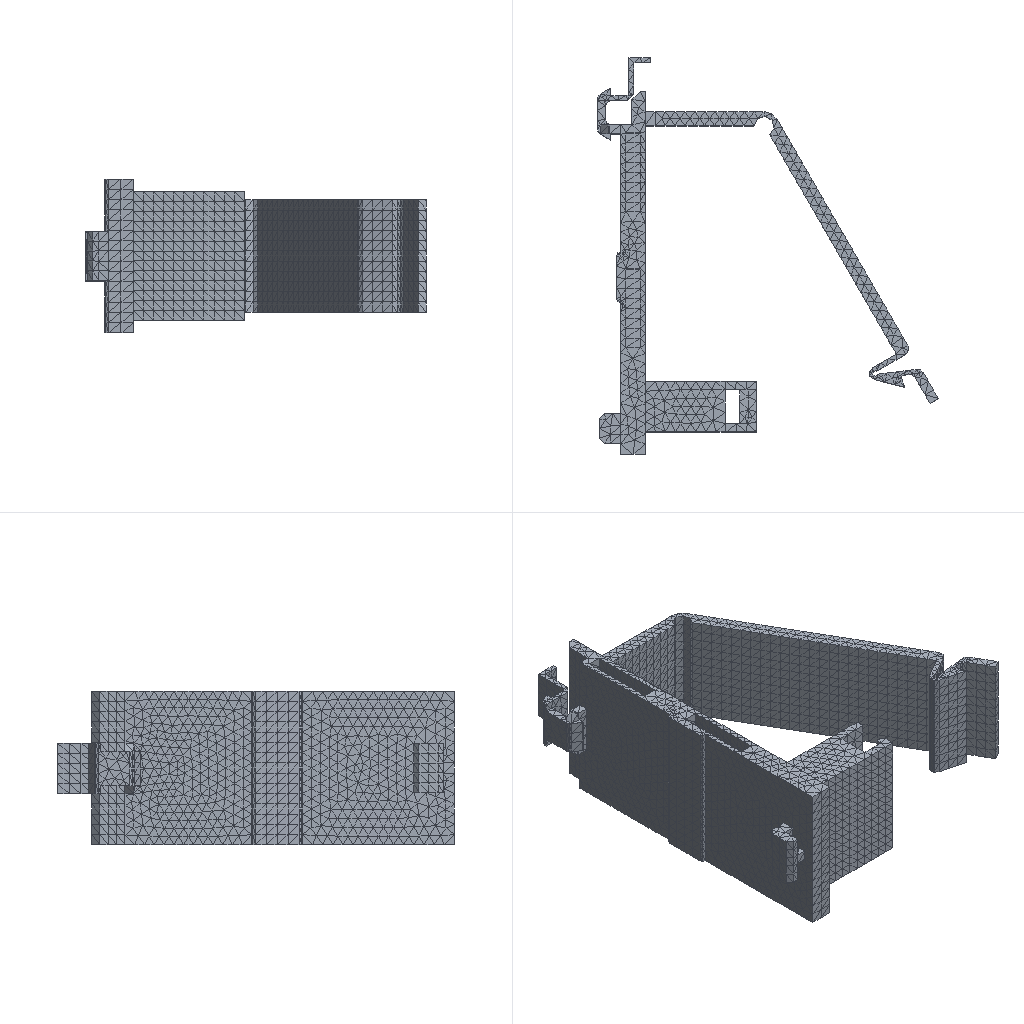Simulation study | abaqus
Set-up summary:
category,name,step,type,value,unit,region
solver,abaqus
solver,version,,,Abaqus/Standard 2020
units,not stated in the deck,,not stated
analysis,deck,,static,static
load_step,Step-1,Step-1,static
load_step,requested,,,1
mesh,nodes,,,5840
mesh,elements,,,20396
element_type,C3D4,,solid,20396
load,load commands in deck,,count,1
bc,support commands in deck,,count,7
material,MATERIAL-1,,in results
check,setup vs results,,match,"per instance, exact: element labels, types and connectivity; labels of the nodes the elements use; coordinates of those nodes at SINGLE_PRECISION in 1 of 1 instance(s)"
Abaqus input file, long lists of numbers shortened:
*Heading
** Job name: Job-1 Model name: Model-1
** Generated by: Abaqus/CAE 2020
*Preprint, echo=NO, model=NO, history=NO, contact=NO
**
** PARTS
**
*Part, name=work
*Node
      1,   3.807,  -1.262,   3.7
      2,   3.807,  -1.262,  -1.3
** (5838 more lines like these left out)
*Element, type=C3D4
    1, 4729, 4730, 4731, 4732
    2, 4733, 4734, 4731, 4729
** (20394 more lines like these left out)
*Nset, nset=Set-1, generate
    1,  5840,     1
*Elset, elset=Set-1, generate
     1,  20396,      1
** Section: Section-1
*Solid Section, elset=Set-1, material=Material-1
,
*End Part
**
**
** ASSEMBLY
**
*Assembly, name=Assembly
**
*Instance, name=work-1, part=work
*End Instance
**
*Node
      1,   16.658,   -4.462,         1.25
*Nset, nset=Set-3, instance=work-1
  104,  105,  106,  107,  108,  109,  110,  111,  112,  113,  114,  115,  116,  117,  118,  119
  120,  121,  122,  123,  205,  206,  209,  210,  217,  218,  219,  220,  223,  224,  225,  226
** (39 more lines like these left out)
*Elset, elset=Set-3, instance=work-1
   136,   425,   620,   758,   814,  1012,  1137,  1196,  1612,  1676,  1698,  1839,  1848,  1909,  1983,  2041
  2067,  2148,  2196,  2292,  2350,  2370,  2664,  2665,  2806,  3074,  3243,  3275,  3323,  3438,  3624,  3682
** (67 more lines like these left out)
*Nset, nset=Set-5
 1,
*Nset, nset=Set-6
 1,
*Nset, nset=m_Set-4
 1,
*Elset, elset=_s_Surf-1_S2, internal, instance=work-1
 6564, 9533, 9553, 9793
*Elset, elset=_s_Surf-1_S4, internal, instance=work-1
  7254,  8519,  9543,  9571,  9627,  9655,  9658,  9760, 14802, 16139, 16232
*Elset, elset=_s_Surf-1_S3, internal, instance=work-1
 9591, 9750, 9766, 9801, 9810
*Elset, elset=_s_Surf-1_S1, internal, instance=work-1
 14791, 15213
*Surface, type=ELEMENT, name=s_Surf-1
_s_Surf-1_S2, S2
_s_Surf-1_S4, S4
_s_Surf-1_S3, S3
_s_Surf-1_S1, S1
*Elset, elset=_s_Surf-2_S3, internal, instance=work-1
  1481,  2183,  6055,  8901,  8902,  9621,  9710,  9794, 10412, 11958, 12014, 12097, 12193, 12241, 12538, 13263
 15121, 15316, 15375, 15410, 15444, 15445, 15446, 15454, 15458, 15477, 15481, 15482, 15502, 15523, 15553, 15556
** (2 more lines like these left out)
*Elset, elset=_s_Surf-2_S2, internal, instance=work-1
  8701,  9544,  9549, 12284, 15347, 15785, 15854
*Elset, elset=_s_Surf-2_S4, internal, instance=work-1
  8908, 12345, 15074, 15408, 15685, 15686
*Surface, type=ELEMENT, name=s_Surf-2
_s_Surf-2_S3, S3
_s_Surf-2_S2, S2
_s_Surf-2_S4, S4
*Elset, elset=_s_Surf-3_S3, internal, instance=work-1
   186,   307,   320,   346,   368,   405,   732,   741,   778,   783,   789,   801,   819,   820,   832,   833
  1380,  1405,  1481,  2042,  2183,  2211,  2278,  2360,  2392,  2395,  2411,  2414,  2422,  2431,  2466,  2467
** (35 more lines like these left out)
*Elset, elset=_s_Surf-3_S2, internal, instance=work-1
  1656,  8701,  9544,  9549, 11553, 11895, 12009, 12233, 12284, 12745, 13031, 14000, 14002, 14131, 15347, 15785
 15854, 16271, 16304, 16542, 19410
*Elset, elset=_s_Surf-3_S4, internal, instance=work-1
  5241,  5366,  8908, 10503, 11551, 11652, 11924, 12345, 12661, 13033, 13185, 15074, 15408, 15425, 15622, 15685
 15686, 16330, 16363, 16391, 16694
*Elset, elset=_s_Surf-3_S1, internal, instance=work-1
 10132, 10498, 10499, 11155, 11770, 11933, 12719, 13337, 13630, 14017, 16260, 16412, 16723
*Surface, type=ELEMENT, name=s_Surf-3
_s_Surf-3_S3, S3
_s_Surf-3_S2, S2
_s_Surf-3_S4, S4
_s_Surf-3_S1, S1
*Elset, elset=_s_Surf-4_S3, internal, instance=work-1
   186,   307,   320,   346,   368,   405,   732,   741,   778,   783,   789,   801,   819,   820,   832,   833
  1380,  1405,  2042,  2211,  2278,  2360,  2392,  2395,  2411,  2414,  2422,  2431,  2466,  2467,  2471,  2472
** (32 more lines like these left out)
*Elset, elset=_s_Surf-4_S2, internal, instance=work-1
  1656, 11553, 11895, 12009, 12233, 12745, 13031, 14000, 14002, 14131, 16271, 16304, 16542, 19410
*Elset, elset=_s_Surf-4_S4, internal, instance=work-1
  5241,  5366, 10503, 11551, 11652, 11924, 12661, 13033, 13185, 15425, 15622, 16330, 16363, 16391, 16694
*Elset, elset=_s_Surf-4_S1, internal, instance=work-1
 10132, 10498, 10499, 11155, 11770, 11933, 12719, 13337, 13630, 14017, 16260, 16412, 16723
*Surface, type=ELEMENT, name=s_Surf-4
_s_Surf-4_S3, S3
_s_Surf-4_S2, S2
_s_Surf-4_S4, S4
_s_Surf-4_S1, S1
*Elset, elset=_s_Surf-5_S3, internal, instance=work-1
   186,   307,   320,   346,   368,   405,   732,   741,   778,   783,   789,   801,   819,   820,   832,   833
  1380,  1405,  1481,  2042,  2183,  2211,  2278,  2360,  2392,  2395,  2411,  2414,  2422,  2431,  2466,  2467
** (35 more lines like these left out)
*Elset, elset=_s_Surf-5_S2, internal, instance=work-1
  1656,  8701,  9544,  9549, 11553, 11895, 12009, 12233, 12284, 12745, 13031, 14000, 14002, 14131, 15347, 15785
 15854, 16271, 16304, 16542, 19410
*Elset, elset=_s_Surf-5_S4, internal, instance=work-1
  5241,  5366,  8908, 10503, 11551, 11652, 11924, 12345, 12661, 13033, 13185, 15074, 15408, 15425, 15622, 15685
 15686, 16330, 16363, 16391, 16694
*Elset, elset=_s_Surf-5_S1, internal, instance=work-1
 10132, 10498, 10499, 11155, 11770, 11933, 12719, 13337, 13630, 14017, 16260, 16412, 16723
*Surface, type=ELEMENT, name=s_Surf-5
_s_Surf-5_S3, S3
_s_Surf-5_S2, S2
_s_Surf-5_S4, S4
_s_Surf-5_S1, S1
** Constraint: Constraint-1
*Coupling, constraint name=Constraint-1, ref node=m_Set-4, surface=s_Surf-5
*Kinematic
*Elset, elset=__Int-1_gcs0_13_S4, internal, instance=work-1
    28,    91,  1847,  2043,  3620,  3893,  5860,  5933,  7082, 19791, 19839, 19908, 19912, 19918, 19932, 19968
 19990, 20005, 20170
*Elset, elset=__Int-1_gcs0_13_S2, internal, instance=work-1
  1608,  2623,  6334, 19907, 19926, 19929, 19942, 20026, 20065, 20068, 20118
*Elset, elset=__Int-1_gcs0_13_S1, internal, instance=work-1
  1850,  2045,  2349,  3618,  3892,  5930, 19953, 19963, 20065
*Elset, elset=__Int-1_gcs0_13_S3, internal, instance=work-1
  2043,  2352,  2995,  3620,  4172,  5933, 10758, 18830, 18924, 19791, 19805, 19808, 19879, 19891, 19912, 19958
 19969, 20005, 20026, 20154, 20175
*Surface, type=ELEMENT, name=_Int-1_gcs0_13, internal
__Int-1_gcs0_13_S4, S4
__Int-1_gcs0_13_S2, S2
__Int-1_gcs0_13_S1, S1
__Int-1_gcs0_13_S3, S3
*Elset, elset=__Int-1_gcs0_31_S3, internal, instance=work-1
   150,  1092,  1641,  2515,  3176,  4288,  4812,  5183,  5382,  5385,  5386,  5977,  6741,  7658,  7882,  8089
  8097, 10686, 11309, 11378, 18115, 18116, 18126, 18142, 18146, 18151, 18154, 18166, 18179, 18184, 18186, 18188
** (1 more lines like these left out)
*Elset, elset=__Int-1_gcs0_31_S4, internal, instance=work-1
   150,  4812,  6741,  7658, 18133, 18165
*Elset, elset=__Int-1_gcs0_31_S2, internal, instance=work-1
 12658, 18119, 18142, 18166
*Elset, elset=__Int-1_gcs0_31_S1, internal, instance=work-1
 18141, 18143, 18169, 18173, 18220
*Surface, type=ELEMENT, name=_Int-1_gcs0_31, internal
__Int-1_gcs0_31_S3, S3
__Int-1_gcs0_31_S4, S4
__Int-1_gcs0_31_S2, S2
__Int-1_gcs0_31_S1, S1
*Elset, elset=__Int-1_gcs0_48_S4, internal, instance=work-1
  625, 3439, 7964, 9232
*Elset, elset=__Int-1_gcs0_48_S3, internal, instance=work-1
 7987, 8059, 9220, 9253, 9256, 9259, 9352
*Elset, elset=__Int-1_gcs0_48_S1, internal, instance=work-1
 9224,
*Surface, type=ELEMENT, name=_Int-1_gcs0_48, internal
__Int-1_gcs0_48_S4, S4
__Int-1_gcs0_48_S3, S3
__Int-1_gcs0_48_S1, S1
*Elset, elset=__Int-1_gcs0_51_S3, internal, instance=work-1
 7932, 7949
*Surface, type=ELEMENT, name=_Int-1_gcs0_51, internal
__Int-1_gcs0_51_S3, S3
*Elset, elset=__Int-1_gcs0_60_S3, internal, instance=work-1
  689, 5132
*Surface, type=ELEMENT, name=_Int-1_gcs0_60, internal
__Int-1_gcs0_60_S3, S3
*Elset, elset=__Int-1_gcs0_65_S3, internal, instance=work-1
  3311,  4775,  7951,  8213,  8231,  8246,  8266,  8273,  8279,  8280, 11068, 11937
*Surface, type=ELEMENT, name=_Int-1_gcs0_65, internal
__Int-1_gcs0_65_S3, S3
*Elset, elset=__Int-1_gcs0_68_S3, internal, instance=work-1
  6145,  7655,  7923,  8062,  8069,  8072,  8074,  8105, 19919
*Elset, elset=__Int-1_gcs0_68_S4, internal, instance=work-1
 7648, 8057, 8087
*Surface, type=ELEMENT, name=_Int-1_gcs0_68, internal
__Int-1_gcs0_68_S3, S3
__Int-1_gcs0_68_S4, S4
*Elset, elset=__Int-1_gcs0_71_S3, internal, instance=work-1
  3012,  3948,  4770,  4773,  7333,  7744,  7746,  7748,  7750,  7758,  7795,  8133,  8182,  8275, 11375, 11431
 14297, 16982, 19820, 19834
*Surface, type=ELEMENT, name=_Int-1_gcs0_71, internal
__Int-1_gcs0_71_S3, S3
*Elset, elset=__Int-1_gcs0_77_S1, internal, instance=work-1
 5330,
*Elset, elset=__Int-1_gcs0_77_S3, internal, instance=work-1
  5331,  7157,  7553,  7820,  7829,  7865,  7866, 11994
*Elset, elset=__Int-1_gcs0_77_S4, internal, instance=work-1
 6113, 6422, 7391, 7468, 7826
*Elset, elset=__Int-1_gcs0_77_S2, internal, instance=work-1
  7066,  7099,  7480,  7817,  7840, 12301
*Surface, type=ELEMENT, name=_Int-1_gcs0_77, internal
__Int-1_gcs0_77_S1, S1
__Int-1_gcs0_77_S3, S3
__Int-1_gcs0_77_S4, S4
__Int-1_gcs0_77_S2, S2
*Elset, elset=__Int-1_gcs0_105_S3, internal, instance=work-1
  1254,  1278,  4655,  8640,  9980,  9983, 10000, 10001, 10105, 14081, 14783, 14793, 14812, 14898, 16859
*Elset, elset=__Int-1_gcs0_105_S2, internal, instance=work-1
 1309, 1400
*Elset, elset=__Int-1_gcs0_105_S1, internal, instance=work-1
  3664,  9929, 14439
*Elset, elset=__Int-1_gcs0_105_S4, internal, instance=work-1
  4501, 13634
*Surface, type=ELEMENT, name=_Int-1_gcs0_105, internal
__Int-1_gcs0_105_S3, S3
__Int-1_gcs0_105_S2, S2
__Int-1_gcs0_105_S4, S4
__Int-1_gcs0_105_S1, S1
*Elset, elset=__Int-1_gcs0_109_S3, internal, instance=work-1
  1342,  1353,  3159,  4391,  4902,  6581,  7990,  9852, 11153, 12632, 14416, 14564, 14627, 14809, 16175, 16178
 16203, 16216, 18307
*Elset, elset=__Int-1_gcs0_109_S4, internal, instance=work-1
  1747,  9559, 12185, 14789, 14792, 16200, 16208, 16218, 20143
*Elset, elset=__Int-1_gcs0_109_S1, internal, instance=work-1
  2218,  4389, 12071, 14668, 14719, 16179, 16201, 16204, 16214
*Elset, elset=__Int-1_gcs0_109_S2, internal, instance=work-1
 15191, 16160, 16186, 16205, 18381, 19782, 20207
*Surface, type=ELEMENT, name=_Int-1_gcs0_109, internal
__Int-1_gcs0_109_S3, S3
__Int-1_gcs0_109_S4, S4
__Int-1_gcs0_109_S2, S2
__Int-1_gcs0_109_S1, S1
*Elset, elset=__Int-1_gcs0_111_S3, internal, instance=work-1
  1313,  1809,  4745, 14050, 15097, 15389, 15424, 15753, 15961, 15968, 15972, 15976, 15993, 15996, 16010, 16040
 16046, 16055, 16076, 16079, 16089, 16741
*Elset, elset=__Int-1_gcs0_111_S2, internal, instance=work-1
  9305, 15966, 15974, 15978, 16006, 16020
*Elset, elset=__Int-1_gcs0_111_S1, internal, instance=work-1
 14482, 15128, 16033, 16051, 16058, 16061, 16899
*Elset, elset=__Int-1_gcs0_111_S4, internal, instance=work-1
 15085, 15989, 16012, 16018, 16022, 16024, 16049, 16056, 19825
*Surface, type=ELEMENT, name=_Int-1_gcs0_111, internal
__Int-1_gcs0_111_S3, S3
__Int-1_gcs0_111_S2, S2
__Int-1_gcs0_111_S4, S4
__Int-1_gcs0_111_S1, S1
*Elset, elset=__Int-1_gcs0_115_S3, internal, instance=work-1
  1811,  1820,  2248,  4059,  4758,  6860,  9540,  9613,  9664, 15048, 15073, 15108, 15132, 15294, 15302, 15303
 15304, 15336, 15345, 15348, 15353, 15357, 15369, 15391, 15393, 15415, 15419, 15421, 15426, 15681, 15750, 15798
** (1 more lines like these left out)
*Elset, elset=__Int-1_gcs0_115_S2, internal, instance=work-1
 2246,
*Surface, type=ELEMENT, name=_Int-1_gcs0_115, internal
__Int-1_gcs0_115_S3, S3
__Int-1_gcs0_115_S2, S2
*Elset, elset=__Int-1_gcs0_117_S1, internal, instance=work-1
  1230,  1233,  1248,  1271,  3297,  4648,  6386,  7533,  9006,  9956, 14462, 14612, 14617, 14644, 14688, 14699
 14701, 14725, 16857, 17858
*Elset, elset=__Int-1_gcs0_117_S3, internal, instance=work-1
  1236,  1246,  1263,  1709,  2444,  2483,  3298,  3300,  3666,  3903,  5816,  6434,  7536,  8247,  8421,  8429
  8940,  9164,  9602,  9934, 10267, 13327, 13683, 14138, 14495, 14577, 14586, 14602, 14615, 14633, 14664, 14665
** (2 more lines like these left out)
*Elset, elset=__Int-1_gcs0_117_S2, internal, instance=work-1
  1243,  9668, 10208, 14149, 14543, 14643, 14685, 14710, 14810, 14877
*Elset, elset=__Int-1_gcs0_117_S4, internal, instance=work-1
  1251,  1258,  1274,  1710,  1730,  1736,  2436,  2479,  2930,  2931,  4652,  6163,  6667,  8586,  9788,  9930
  9938,  9947, 10052, 10101, 14412, 14461, 14583, 14608, 14618, 14626, 14631, 14648, 14653, 14654, 14663, 14680
** (1 more lines like these left out)
*Surface, type=ELEMENT, name=_Int-1_gcs0_117, internal
__Int-1_gcs0_117_S1, S1
__Int-1_gcs0_117_S3, S3
__Int-1_gcs0_117_S2, S2
__Int-1_gcs0_117_S4, S4
*Elset, elset=__Int-1_gcs0_119_S3, internal, instance=work-1
  2201,  4167,  5370,  5374,  5424,  5471,  5941,  6551,  9523, 10229, 10287, 10291, 10321, 10402, 10408, 10423
 12354, 12364, 12382, 13360, 13495, 13644, 13708, 13709, 13787, 13800, 14285, 14287, 14303, 14308, 14323, 14328
** (1 more lines like these left out)
*Surface, type=ELEMENT, name=_Int-1_gcs0_119, internal
__Int-1_gcs0_119_S3, S3
*Elset, elset=__Int-1_gcs0_121_S3, internal, instance=work-1
  6369, 11889, 11975, 11979, 12001, 12095, 12099, 12130, 12133, 12154, 12177, 12190, 12245, 12297, 12307, 12339
 16280, 16300, 16341, 16430, 16464, 16469, 16495, 16519
*Elset, elset=__Int-1_gcs0_121_S4, internal, instance=work-1
  7223, 11838, 11894, 12057, 12098, 12135, 12152, 12256, 12273, 12330, 16451
*Elset, elset=__Int-1_gcs0_121_S2, internal, instance=work-1
 12114, 12239, 16233, 16281
*Elset, elset=__Int-1_gcs0_121_S1, internal, instance=work-1
 12291, 12328, 16356, 16414, 16433
*Surface, type=ELEMENT, name=_Int-1_gcs0_121, internal
__Int-1_gcs0_121_S3, S3
__Int-1_gcs0_121_S4, S4
__Int-1_gcs0_121_S2, S2
__Int-1_gcs0_121_S1, S1
*Elset, elset=__Int-1_gcs0_125_S1, internal, instance=work-1
  1240,  9266, 10091, 10128, 10228, 14434, 14460, 14702, 14715
*Elset, elset=__Int-1_gcs0_125_S3, internal, instance=work-1
  1275,  3296,  4498,  4499,  6125,  6278,  8917,  9558,  9805,  9982, 10051, 10068, 10070, 10076, 10083, 10087
 10098, 10099, 10115, 10123, 10143, 10157, 10207, 14146, 14491, 14517, 14673, 14679, 14691, 14727, 14766, 15648
*Elset, elset=__Int-1_gcs0_125_S4, internal, instance=work-1
 4529,
*Elset, elset=__Int-1_gcs0_125_S2, internal, instance=work-1
 10112, 14718
*Surface, type=ELEMENT, name=_Int-1_gcs0_125, internal
__Int-1_gcs0_125_S1, S1
__Int-1_gcs0_125_S3, S3
__Int-1_gcs0_125_S4, S4
__Int-1_gcs0_125_S2, S2
*Elset, elset=__Int-1_gcs0_128_S3, internal, instance=work-1
   358,  3627,  4106,  6086,  8077, 11999, 12007, 12013, 12079, 12086, 12197, 13332, 13489, 13626, 14066, 14689
 14734, 15431, 15475, 16238, 16276, 16290, 16297, 16299, 16310, 16328, 16334, 16369, 16378, 16381, 16388, 16418
** (2 more lines like these left out)
*Elset, elset=__Int-1_gcs0_128_S2, internal, instance=work-1
  6342, 11012, 12081, 12136, 12159, 16355, 16358, 16370, 16383, 16390, 16395, 16435, 16455, 16475, 16488, 16503
 16504, 16510, 16512, 16547
*Elset, elset=__Int-1_gcs0_128_S1, internal, instance=work-1
 12104, 16172, 16272, 16273, 16279, 16318, 16322, 16327, 16329, 16340, 16351, 16368, 16424, 16473, 16532, 16534
 16561,
*Elset, elset=__Int-1_gcs0_128_S4, internal, instance=work-1
 12129, 12161, 12178, 12186, 12718, 12753, 12896, 16251, 16262, 16265, 16292, 16321, 16332, 16376, 16393, 16397
 16423, 16426, 16441, 16442, 16515, 16524, 16569, 16721
*Surface, type=ELEMENT, name=_Int-1_gcs0_128, internal
__Int-1_gcs0_128_S3, S3
__Int-1_gcs0_128_S2, S2
__Int-1_gcs0_128_S4, S4
__Int-1_gcs0_128_S1, S1
*End Assembly
**
** MATERIALS
**
*Material, name=Material-1
*Density
 1.15e-09,
*Elastic
1060., 0.35
**
** INTERACTION PROPERTIES
**
*Surface Interaction, name=IntProp-1
1.,
*Friction, slip tolerance=0.005
 0.4,
*Surface Behavior, pressure-overclosure=HARD
**
** INTERACTIONS
**
** Interaction: Int-1
*Contact
*Contact Inclusions, ALL EXTERIOR
*Contact Property Assignment
 ,  , IntProp-1
*Surface Property Assignment, property=GEOMETRIC CORRECTION
_Int-1_gcs0_13, Circumferential, 2.457, -21.462, -26.165,  2.457, -21.462, -27.165
_Int-1_gcs0_31, Circumferential, 2.457, -17.162, 28.665,  2.457, -17.162, 29.665
_Int-1_gcs0_48, Circumferential, 1.507, -3.762, 28.665,  1.507, -3.762, 29.665
_Int-1_gcs0_51, Circumferential, 1.39, 53.489, 3.5,  1.39, 54.489, 3.5
_Int-1_gcs0_60, Circumferential, 1.39, -75.198, -1.1,  1.39, -76.198, -1.1
_Int-1_gcs0_65, Circumferential, 1.507, -2.362, -26.165,  1.507, -2.362, -27.165
_Int-1_gcs0_68, Circumferential, 0.707, -4.758, -26.165,  0.707, -4.758, -27.165
_Int-1_gcs0_71, Circumferential, 0.707, -1.644, 28.665,  0.707, -1.644, 29.665
_Int-1_gcs0_77, Circumferential, 3.007, -1.062, 3.7,  3.007, -1.062, 4.7
_Int-1_gcs0_105, Circumferential, 27.676, -28.847, -26.165,  27.676, -28.847, -27.165
_Int-1_gcs0_109, Circumferential, 30.426, -29.196, 6.35,  30.426, -29.196, 7.35
_Int-1_gcs0_111, Circumferential, 31.067, -29.52, 6.35,  31.067, -29.52, 5.35
_Int-1_gcs0_115, Circumferential, 31.874, -29.018, 6.35,  31.874, -29.018, 7.35
_Int-1_gcs0_117, Circumferential, 27.64, -28.829, 6.35,  27.64, -28.829, 7.35
_Int-1_gcs0_119, Circumferential, 30.376, -26.423, -26.165,  30.376, -26.423, -27.165
_Int-1_gcs0_121, Circumferential, 16.657, -4.462, 6.35,  16.657, -4.462, 5.35
_Int-1_gcs0_125, Circumferential, 27.651, -28.804, -26.165,  27.651, -28.804, -27.165
_Int-1_gcs0_128, Circumferential, 16.665, -4.412, 4.3,  16.665, -4.412, 5.3
** ----------------------------------------------------------------
**
** STEP: Step-1
**
*Step, name=Step-1, nlgeom=YES, inc=10000
*Static, stabilize=0.0002, allsdtol=0.05, continue=NO
0.01, 1., 1e-05, 1.
**
** BOUNDARY CONDITIONS
**
** Name: fixed Type: 对称/反对称/完全固定
*Boundary
Set-3, ENCASTRE
** Name: weiyi Type: Displacement/Rotation angle
*Boundary
Set-6, 1, 1
Set-6, 2, 2
Set-6, 3, 3
Set-6, 4, 4
Set-6, 5, 5
Set-6, 6, 6, -31.7
**
** OUTPUT REQUESTS
**
*Restart, write, number interval=1, time marks=NO
**
** FIELD OUTPUT: F-Output-1
**
*Output, field
*Node Output
RF, U, V
*Element Output, directions=YES
E, LE, MISES, PE, PEEQ, S
*Contact Output
CDISP, CSTRESS
**
** HISTORY OUTPUT: H-Output-1
**
*Output, history, number interval=1000, time marks=NO
*Node Output, nset=m_Set-4
RF1, RF2, RF3, RM1, RM2, RM3, U1, U2
U3, UR1, UR2, UR3
*End Step
Results summary:
result,step,,partial,increments=30 time=0.01707/1.0
result,analysis,,,static
result,last_loadstep,,,1
result,primary field,,,U
result,reaction total,,FX,-0.2284,model units
result,reaction total,,FY,-1.237,model units
result,reaction total,,FZ,-0.1832,model units